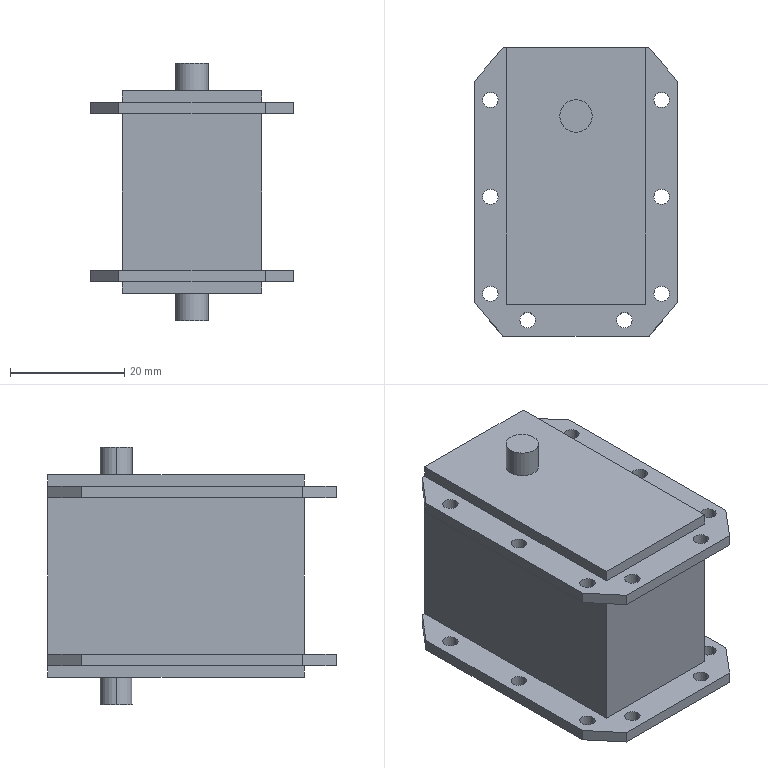Part | SolidWorks | features BaseBody 1, ICE 1 | 1 solid | 68 faces | box 35.6 x 50.6 x 45.2 mm | volume 41620 mm3 | cylinder 36 | plane 32 | commonest cylinder face diameters 2.7 x32 5.7 x4